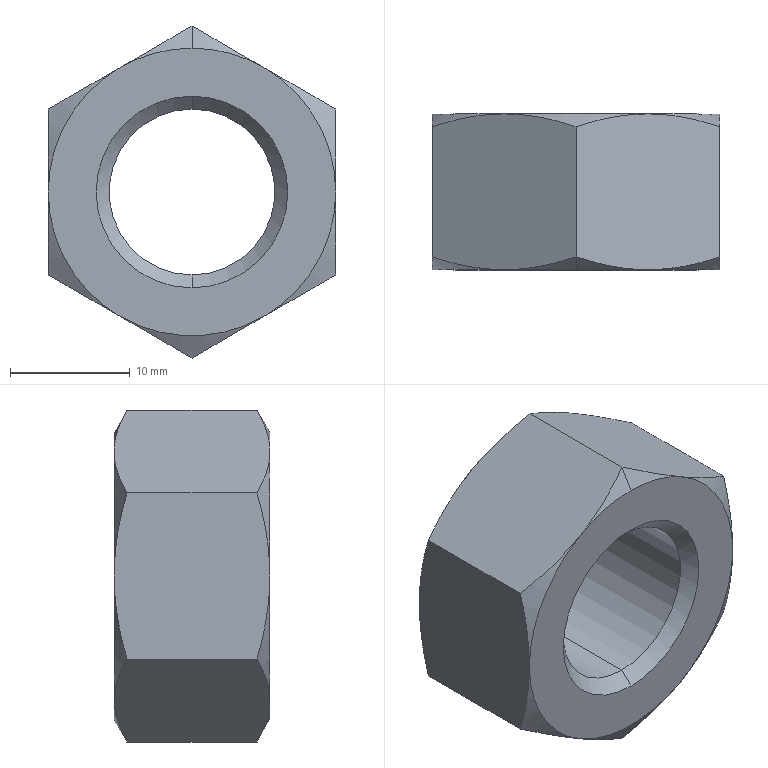Part | STEP file | 1 solid | 28 faces | box 24 x 13 x 27.713 mm | volume 4447 mm3 | cone 18 | plane 8 | cylinder 2 | commonest cylinder face diameters 13.835 x2